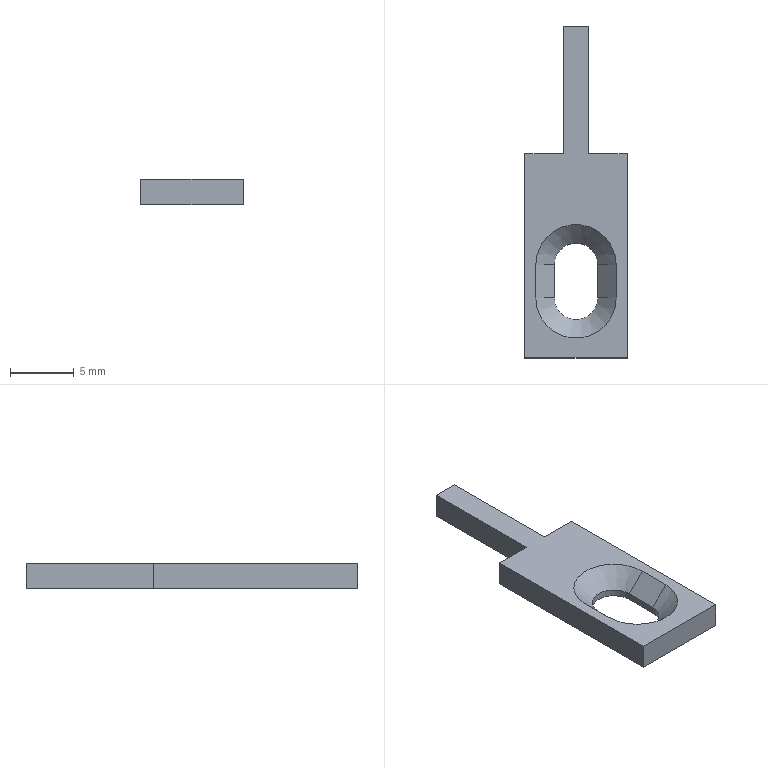Part | NX | features BREP 1 | 1 solid | 18 faces | box 8 x 26 x 2 mm | volume 240.274 mm3 | plane 14 | cone 2 | cylinder 2 | commonest cylinder face diameters 3.4 x2
STEP:
#1=CARTESIAN_POINT('',(-3.15,-3.3,2.));
#2=VERTEX_POINT('',#1);
#3=CARTESIAN_POINT('',(-1.7,-3.3,0.55));
#4=VERTEX_POINT('',#3);
#5=CARTESIAN_POINT('',(0.,-3.3,-1.15));
#6=DIRECTION('',(0.7071,0.,-0.7071));
#7=VECTOR('',#6,1000.);
#8=LINE('',#5,#7);
#9=EDGE_CURVE('',#2,#4,#8,.T.);
#10=ORIENTED_EDGE('',*,*,#9,.T.);
#11=CARTESIAN_POINT('',(-1.7,-0.7,0.55));
#12=VERTEX_POINT('',#11);
#13=CARTESIAN_POINT('',(-1.7,-0.7,0.55));
#14=DIRECTION('',(0.,-1.,0.));
#15=VECTOR('',#14,1000.);
#16=LINE('',#13,#15);
#17=EDGE_CURVE('',#12,#4,#16,.T.);
#18=ORIENTED_EDGE('',*,*,#17,.F.);
#19=CARTESIAN_POINT('',(-3.15,-0.7,2.));
#20=VERTEX_POINT('',#19);
#21=CARTESIAN_POINT('',(0.,-0.7,-1.15));
#22=DIRECTION('',(-0.7071,0.,0.7071));
#23=VECTOR('',#22,1000.);
#24=LINE('',#21,#23);
#25=EDGE_CURVE('',#12,#20,#24,.T.);
#26=ORIENTED_EDGE('',*,*,#25,.T.);
#27=CARTESIAN_POINT('',(-3.15,-0.7,2.));
#28=DIRECTION('',(0.,-1.,0.));
#29=VECTOR('',#28,1000.);
#30=LINE('',#27,#29);
#31=EDGE_CURVE('',#20,#2,#30,.T.);
#32=ORIENTED_EDGE('',*,*,#31,.T.);
#33=EDGE_LOOP('',(#10,#18,#26,#32));
#34=FACE_BOUND('',#33,.T.);
#35=CARTESIAN_POINT('',(0.,-0.7,-1.15));
#36=DIRECTION('',(-0.7071,0.,-0.7071));
#37=DIRECTION('',(-0.7071,0.,0.7071));
#38=AXIS2_PLACEMENT_3D('',#35,#36,#37);
#39=PLANE('',#38);
#40=ADVANCED_FACE('',(#34),#39,.F.);
#41=CARTESIAN_POINT('',(3.15,-3.3,2.));
#42=VERTEX_POINT('',#41);
#43=CARTESIAN_POINT('',(1.7,-3.3,0.55));
#44=VERTEX_POINT('',#43);
#45=CARTESIAN_POINT('',(1.7,-3.3,0.55));
#46=DIRECTION('',(-0.7071,0.,-0.7071));
#47=VECTOR('',#46,1000.);
#48=LINE('',#45,#47);
#49=EDGE_CURVE('',#42,#44,#48,.T.);
#50=ORIENTED_EDGE('',*,*,#49,.F.);
#51=CARTESIAN_POINT('',(3.15,-0.7,2.));
#52=VERTEX_POINT('',#51);
#53=CARTESIAN_POINT('',(3.15,-0.7,2.));
#54=DIRECTION('',(0.,-1.,0.));
#55=VECTOR('',#54,1000.);
#56=LINE('',#53,#55);
#57=EDGE_CURVE('',#52,#42,#56,.T.);
#58=ORIENTED_EDGE('',*,*,#57,.F.);
#59=CARTESIAN_POINT('',(1.7,-0.7,0.55));
#60=VERTEX_POINT('',#59);
#61=CARTESIAN_POINT('',(1.7,-0.7,0.55));
#62=DIRECTION('',(-0.7071,0.,-0.7071));
#63=VECTOR('',#62,1000.);
#64=LINE('',#61,#63);
#65=EDGE_CURVE('',#52,#60,#64,.T.);
#66=ORIENTED_EDGE('',*,*,#65,.T.);
#67=CARTESIAN_POINT('',(1.7,-0.7,0.55));
#68=DIRECTION('',(0.,-1.,0.));
#69=VECTOR('',#68,1000.);
#70=LINE('',#67,#69);
#71=EDGE_CURVE('',#60,#44,#70,.T.);
#72=ORIENTED_EDGE('',*,*,#71,.T.);
#73=EDGE_LOOP('',(#50,#58,#66,#72));
#74=FACE_BOUND('',#73,.T.);
#75=CARTESIAN_POINT('',(1.7,-0.7,0.55));
#76=DIRECTION('',(-0.7071,0.,0.7071));
#77=DIRECTION('',(0.7071,0.,0.7071));
#78=AXIS2_PLACEMENT_3D('',#75,#76,#77);
#79=PLANE('',#78);
#80=ADVANCED_FACE('',(#74),#79,.T.);
#81=CARTESIAN_POINT('',(0.,-0.7,0.55));
#82=DIRECTION('',(0.,0.,1.));
#83=DIRECTION('',(1.,0.,0.));
#84=AXIS2_PLACEMENT_3D('',#81,#82,#83);
#85=CIRCLE('',#84,1.7);
#86=EDGE_CURVE('',#60,#12,#85,.T.);
#87=ORIENTED_EDGE('',*,*,#86,.F.);
#88=ORIENTED_EDGE('',*,*,#65,.F.);
#89=CARTESIAN_POINT('',(0.,-0.7,2.));
#90=DIRECTION('',(0.,0.,1.));
#91=DIRECTION('',(1.,0.,0.));
#92=AXIS2_PLACEMENT_3D('',#89,#90,#91);
#93=CIRCLE('',#92,3.15);
#94=EDGE_CURVE('',#52,#20,#93,.T.);
#95=ORIENTED_EDGE('',*,*,#94,.T.);
#96=ORIENTED_EDGE('',*,*,#25,.F.);
#97=EDGE_LOOP('',(#87,#88,#95,#96));
#98=FACE_BOUND('',#97,.T.);
#99=CARTESIAN_POINT('',(0.,-0.7,2.));
#100=DIRECTION('',(0.,0.,1.));
#101=DIRECTION('',(1.,0.,0.));
#102=AXIS2_PLACEMENT_3D('',#99,#100,#101);
#103=CONICAL_SURFACE('',#102,3.15,0.7854);
#104=ADVANCED_FACE('',(#98),#103,.F.);
#105=CARTESIAN_POINT('',(0.,-3.3,2.));
#106=DIRECTION('',(0.,0.,1.));
#107=DIRECTION('',(1.,0.,0.));
#108=AXIS2_PLACEMENT_3D('',#105,#106,#107);
#109=CIRCLE('',#108,3.15);
#110=EDGE_CURVE('',#2,#42,#109,.T.);
#111=ORIENTED_EDGE('',*,*,#110,.T.);
#112=ORIENTED_EDGE('',*,*,#49,.T.);
#113=CARTESIAN_POINT('',(0.,-3.3,0.55));
#114=DIRECTION('',(0.,0.,1.));
#115=DIRECTION('',(1.,0.,0.));
#116=AXIS2_PLACEMENT_3D('',#113,#114,#115);
#117=CIRCLE('',#116,1.7);
#118=EDGE_CURVE('',#4,#44,#117,.T.);
#119=ORIENTED_EDGE('',*,*,#118,.F.);
#120=ORIENTED_EDGE('',*,*,#9,.F.);
#121=EDGE_LOOP('',(#111,#112,#119,#120));
#122=FACE_BOUND('',#121,.T.);
#123=CARTESIAN_POINT('',(0.,-3.3,2.));
#124=DIRECTION('',(0.,0.,1.));
#125=DIRECTION('',(1.,0.,0.));
#126=AXIS2_PLACEMENT_3D('',#123,#124,#125);
#127=CONICAL_SURFACE('',#126,3.15,0.7854);
#128=ADVANCED_FACE('',(#122),#127,.F.);
#129=CARTESIAN_POINT('',(1.7,-0.7,0.));
#130=VERTEX_POINT('',#129);
#131=CARTESIAN_POINT('',(1.7,-3.3,0.));
#132=VERTEX_POINT('',#131);
#133=CARTESIAN_POINT('',(1.7,0.,0.));
#134=DIRECTION('',(0.,-1.,0.));
#135=VECTOR('',#134,1000.);
#136=LINE('',#133,#135);
#137=EDGE_CURVE('',#130,#132,#136,.T.);
#138=ORIENTED_EDGE('',*,*,#137,.T.);
#139=CARTESIAN_POINT('',(1.7,-3.3,-16.));
#140=DIRECTION('',(0.,0.,-1.));
#141=VECTOR('',#140,1000.);
#142=LINE('',#139,#141);
#143=EDGE_CURVE('',#44,#132,#142,.T.);
#144=ORIENTED_EDGE('',*,*,#143,.F.);
#145=ORIENTED_EDGE('',*,*,#71,.F.);
#146=CARTESIAN_POINT('',(1.7,-0.7,-16.));
#147=DIRECTION('',(0.,0.,-1.));
#148=VECTOR('',#147,1000.);
#149=LINE('',#146,#148);
#150=EDGE_CURVE('',#60,#130,#149,.T.);
#151=ORIENTED_EDGE('',*,*,#150,.T.);
#152=EDGE_LOOP('',(#138,#144,#145,#151));
#153=FACE_BOUND('',#152,.T.);
#154=CARTESIAN_POINT('',(1.7,-0.7,-16.));
#155=DIRECTION('',(-1.,0.,0.));
#156=DIRECTION('',(0.,-1.,0.));
#157=AXIS2_PLACEMENT_3D('',#154,#155,#156);
#158=PLANE('',#157);
#159=ADVANCED_FACE('',(#153),#158,.T.);
#160=CARTESIAN_POINT('',(-1.7,-0.7,0.));
#161=VERTEX_POINT('',#160);
#162=CARTESIAN_POINT('',(-1.7,-0.7,2.));
#163=DIRECTION('',(0.,0.,1.));
#164=VECTOR('',#163,1000.);
#165=LINE('',#162,#164);
#166=EDGE_CURVE('',#161,#12,#165,.T.);
#167=ORIENTED_EDGE('',*,*,#166,.T.);
#168=ORIENTED_EDGE('',*,*,#17,.T.);
#169=CARTESIAN_POINT('',(-1.7,-3.3,0.));
#170=VERTEX_POINT('',#169);
#171=CARTESIAN_POINT('',(-1.7,-3.3,2.));
#172=DIRECTION('',(0.,0.,-1.));
#173=VECTOR('',#172,1000.);
#174=LINE('',#171,#173);
#175=EDGE_CURVE('',#4,#170,#174,.T.);
#176=ORIENTED_EDGE('',*,*,#175,.T.);
#177=CARTESIAN_POINT('',(-1.7,0.,0.));
#178=DIRECTION('',(0.,-1.,0.));
#179=VECTOR('',#178,1000.);
#180=LINE('',#177,#179);
#181=EDGE_CURVE('',#161,#170,#180,.T.);
#182=ORIENTED_EDGE('',*,*,#181,.F.);
#183=EDGE_LOOP('',(#167,#168,#176,#182));
#184=FACE_BOUND('',#183,.T.);
#185=CARTESIAN_POINT('',(-1.7,-0.7,2.));
#186=DIRECTION('',(-1.,0.,0.));
#187=DIRECTION('',(0.,-1.,0.));
#188=AXIS2_PLACEMENT_3D('',#185,#186,#187);
#189=PLANE('',#188);
#190=ADVANCED_FACE('',(#184),#189,.F.);
#191=ORIENTED_EDGE('',*,*,#175,.F.);
#192=ORIENTED_EDGE('',*,*,#118,.T.);
#193=ORIENTED_EDGE('',*,*,#143,.T.);
#194=CARTESIAN_POINT('',(0.,-3.3,0.));
#195=DIRECTION('',(0.,0.,1.));
#196=DIRECTION('',(1.,0.,0.));
#197=AXIS2_PLACEMENT_3D('',#194,#195,#196);
#198=CIRCLE('',#197,1.7);
#199=EDGE_CURVE('',#170,#132,#198,.T.);
#200=ORIENTED_EDGE('',*,*,#199,.F.);
#201=EDGE_LOOP('',(#191,#192,#193,#200));
#202=FACE_BOUND('',#201,.T.);
#203=CARTESIAN_POINT('',(0.,-3.3,2.));
#204=DIRECTION('',(0.,0.,1.));
#205=DIRECTION('',(1.,0.,0.));
#206=AXIS2_PLACEMENT_3D('',#203,#204,#205);
#207=CYLINDRICAL_SURFACE('',#206,1.7);
#208=ADVANCED_FACE('',(#202),#207,.F.);
#209=ORIENTED_EDGE('',*,*,#150,.F.);
#210=ORIENTED_EDGE('',*,*,#86,.T.);
#211=ORIENTED_EDGE('',*,*,#166,.F.);
#212=CARTESIAN_POINT('',(0.,-0.7,0.));
#213=DIRECTION('',(0.,0.,1.));
#214=DIRECTION('',(1.,0.,0.));
#215=AXIS2_PLACEMENT_3D('',#212,#213,#214);
#216=CIRCLE('',#215,1.7);
#217=EDGE_CURVE('',#130,#161,#216,.T.);
#218=ORIENTED_EDGE('',*,*,#217,.F.);
#219=EDGE_LOOP('',(#209,#210,#211,#218));
#220=FACE_BOUND('',#219,.T.);
#221=CARTESIAN_POINT('',(0.,-0.7,2.));
#222=DIRECTION('',(0.,0.,1.));
#223=DIRECTION('',(1.,0.,0.));
#224=AXIS2_PLACEMENT_3D('',#221,#222,#223);
#225=CYLINDRICAL_SURFACE('',#224,1.7);
#226=ADVANCED_FACE('',(#220),#225,.F.);
#227=CARTESIAN_POINT('',(4.,8.,0.));
#228=VERTEX_POINT('',#227);
#229=CARTESIAN_POINT('',(1.,8.,0.));
#230=VERTEX_POINT('',#229);
#231=CARTESIAN_POINT('',(1.,8.,0.));
#232=DIRECTION('',(-1.,0.,0.));
#233=VECTOR('',#232,1000.);
#234=LINE('',#231,#233);
#235=EDGE_CURVE('',#228,#230,#234,.T.);
#236=ORIENTED_EDGE('',*,*,#235,.F.);
#237=CARTESIAN_POINT('',(4.,-8.,0.));
#238=VERTEX_POINT('',#237);
#239=CARTESIAN_POINT('',(4.,-8.,0.));
#240=DIRECTION('',(0.,1.,0.));
#241=VECTOR('',#240,1000.);
#242=LINE('',#239,#241);
#243=EDGE_CURVE('',#238,#228,#242,.T.);
#244=ORIENTED_EDGE('',*,*,#243,.F.);
#245=CARTESIAN_POINT('',(-4.,-8.,0.));
#246=VERTEX_POINT('',#245);
#247=CARTESIAN_POINT('',(-4.,-8.,0.));
#248=DIRECTION('',(1.,0.,0.));
#249=VECTOR('',#248,1000.);
#250=LINE('',#247,#249);
#251=EDGE_CURVE('',#246,#238,#250,.T.);
#252=ORIENTED_EDGE('',*,*,#251,.F.);
#253=CARTESIAN_POINT('',(-4.,8.,0.));
#254=VERTEX_POINT('',#253);
#255=CARTESIAN_POINT('',(-4.,-8.,0.));
#256=DIRECTION('',(0.,-1.,0.));
#257=VECTOR('',#256,1000.);
#258=LINE('',#255,#257);
#259=EDGE_CURVE('',#254,#246,#258,.T.);
#260=ORIENTED_EDGE('',*,*,#259,.F.);
#261=CARTESIAN_POINT('',(-1.,8.,0.));
#262=VERTEX_POINT('',#261);
#263=CARTESIAN_POINT('',(-4.,8.,0.));
#264=DIRECTION('',(-1.,0.,0.));
#265=VECTOR('',#264,1000.);
#266=LINE('',#263,#265);
#267=EDGE_CURVE('',#262,#254,#266,.T.);
#268=ORIENTED_EDGE('',*,*,#267,.F.);
#269=CARTESIAN_POINT('',(-1.,18.,0.));
#270=VERTEX_POINT('',#269);
#271=CARTESIAN_POINT('',(-1.,18.,0.));
#272=DIRECTION('',(0.,-1.,0.));
#273=VECTOR('',#272,1000.);
#274=LINE('',#271,#273);
#275=EDGE_CURVE('',#270,#262,#274,.T.);
#276=ORIENTED_EDGE('',*,*,#275,.F.);
#277=CARTESIAN_POINT('',(1.,18.,0.));
#278=VERTEX_POINT('',#277);
#279=CARTESIAN_POINT('',(1.,18.,0.));
#280=DIRECTION('',(-1.,0.,0.));
#281=VECTOR('',#280,1000.);
#282=LINE('',#279,#281);
#283=EDGE_CURVE('',#278,#270,#282,.T.);
#284=ORIENTED_EDGE('',*,*,#283,.F.);
#285=CARTESIAN_POINT('',(1.,18.,0.));
#286=DIRECTION('',(0.,1.,0.));
#287=VECTOR('',#286,1000.);
#288=LINE('',#285,#287);
#289=EDGE_CURVE('',#230,#278,#288,.T.);
#290=ORIENTED_EDGE('',*,*,#289,.F.);
#291=EDGE_LOOP('',(#236,#244,#252,#260,#268,#276,#284,#290));
#292=FACE_BOUND('',#291,.T.);
#293=ORIENTED_EDGE('',*,*,#217,.T.);
#294=ORIENTED_EDGE('',*,*,#181,.T.);
#295=ORIENTED_EDGE('',*,*,#199,.T.);
#296=ORIENTED_EDGE('',*,*,#137,.F.);
#297=EDGE_LOOP('',(#293,#294,#295,#296));
#298=FACE_BOUND('',#297,.T.);
#299=CARTESIAN_POINT('',(0.,0.,0.));
#300=DIRECTION('',(0.,0.,1.));
#301=DIRECTION('',(1.,0.,0.));
#302=AXIS2_PLACEMENT_3D('',#299,#300,#301);
#303=PLANE('',#302);
#304=ADVANCED_FACE('',(#292,#298),#303,.F.);
#305=CARTESIAN_POINT('',(4.,8.,2.));
#306=VERTEX_POINT('',#305);
#307=CARTESIAN_POINT('',(1.,8.,2.));
#308=VERTEX_POINT('',#307);
#309=CARTESIAN_POINT('',(1.,8.,2.));
#310=DIRECTION('',(-1.,0.,0.));
#311=VECTOR('',#310,1000.);
#312=LINE('',#309,#311);
#313=EDGE_CURVE('',#306,#308,#312,.T.);
#314=ORIENTED_EDGE('',*,*,#313,.T.);
#315=CARTESIAN_POINT('',(1.,18.,2.));
#316=VERTEX_POINT('',#315);
#317=CARTESIAN_POINT('',(1.,18.,2.));
#318=DIRECTION('',(0.,1.,0.));
#319=VECTOR('',#318,1000.);
#320=LINE('',#317,#319);
#321=EDGE_CURVE('',#308,#316,#320,.T.);
#322=ORIENTED_EDGE('',*,*,#321,.T.);
#323=CARTESIAN_POINT('',(-1.,18.,2.));
#324=VERTEX_POINT('',#323);
#325=CARTESIAN_POINT('',(1.,18.,2.));
#326=DIRECTION('',(-1.,0.,0.));
#327=VECTOR('',#326,1000.);
#328=LINE('',#325,#327);
#329=EDGE_CURVE('',#316,#324,#328,.T.);
#330=ORIENTED_EDGE('',*,*,#329,.T.);
#331=CARTESIAN_POINT('',(-1.,8.,2.));
#332=VERTEX_POINT('',#331);
#333=CARTESIAN_POINT('',(-1.,18.,2.));
#334=DIRECTION('',(0.,-1.,0.));
#335=VECTOR('',#334,1000.);
#336=LINE('',#333,#335);
#337=EDGE_CURVE('',#324,#332,#336,.T.);
#338=ORIENTED_EDGE('',*,*,#337,.T.);
#339=CARTESIAN_POINT('',(-4.,8.,2.));
#340=VERTEX_POINT('',#339);
#341=CARTESIAN_POINT('',(-4.,8.,2.));
#342=DIRECTION('',(-1.,0.,0.));
#343=VECTOR('',#342,1000.);
#344=LINE('',#341,#343);
#345=EDGE_CURVE('',#332,#340,#344,.T.);
#346=ORIENTED_EDGE('',*,*,#345,.T.);
#347=CARTESIAN_POINT('',(-4.,-8.,2.));
#348=VERTEX_POINT('',#347);
#349=CARTESIAN_POINT('',(-4.,-8.,2.));
#350=DIRECTION('',(0.,-1.,0.));
#351=VECTOR('',#350,1000.);
#352=LINE('',#349,#351);
#353=EDGE_CURVE('',#340,#348,#352,.T.);
#354=ORIENTED_EDGE('',*,*,#353,.T.);
#355=CARTESIAN_POINT('',(4.,-8.,2.));
#356=VERTEX_POINT('',#355);
#357=CARTESIAN_POINT('',(-4.,-8.,2.));
#358=DIRECTION('',(1.,0.,0.));
#359=VECTOR('',#358,1000.);
#360=LINE('',#357,#359);
#361=EDGE_CURVE('',#348,#356,#360,.T.);
#362=ORIENTED_EDGE('',*,*,#361,.T.);
#363=CARTESIAN_POINT('',(4.,-8.,2.));
#364=DIRECTION('',(0.,1.,0.));
#365=VECTOR('',#364,1000.);
#366=LINE('',#363,#365);
#367=EDGE_CURVE('',#356,#306,#366,.T.);
#368=ORIENTED_EDGE('',*,*,#367,.T.);
#369=EDGE_LOOP('',(#314,#322,#330,#338,#346,#354,#362,#368));
#370=FACE_BOUND('',#369,.T.);
#371=ORIENTED_EDGE('',*,*,#31,.F.);
#372=ORIENTED_EDGE('',*,*,#94,.F.);
#373=ORIENTED_EDGE('',*,*,#57,.T.);
#374=ORIENTED_EDGE('',*,*,#110,.F.);
#375=EDGE_LOOP('',(#371,#372,#373,#374));
#376=FACE_BOUND('',#375,.T.);
#377=CARTESIAN_POINT('',(0.,0.,2.));
#378=DIRECTION('',(0.,0.,1.));
#379=DIRECTION('',(1.,0.,0.));
#380=AXIS2_PLACEMENT_3D('',#377,#378,#379);
#381=PLANE('',#380);
#382=ADVANCED_FACE('',(#370,#376),#381,.T.);
#383=ORIENTED_EDGE('',*,*,#243,.T.);
#384=CARTESIAN_POINT('',(4.,8.,2.));
#385=DIRECTION('',(0.,0.,-1.));
#386=VECTOR('',#385,1000.);
#387=LINE('',#384,#386);
#388=EDGE_CURVE('',#306,#228,#387,.T.);
#389=ORIENTED_EDGE('',*,*,#388,.F.);
#390=ORIENTED_EDGE('',*,*,#367,.F.);
#391=CARTESIAN_POINT('',(4.,-8.,2.));
#392=DIRECTION('',(0.,0.,-1.));
#393=VECTOR('',#392,1000.);
#394=LINE('',#391,#393);
#395=EDGE_CURVE('',#356,#238,#394,.T.);
#396=ORIENTED_EDGE('',*,*,#395,.T.);
#397=EDGE_LOOP('',(#383,#389,#390,#396));
#398=FACE_BOUND('',#397,.T.);
#399=CARTESIAN_POINT('',(4.,-8.,2.));
#400=DIRECTION('',(-1.,0.,0.));
#401=DIRECTION('',(0.,0.,1.));
#402=AXIS2_PLACEMENT_3D('',#399,#400,#401);
#403=PLANE('',#402);
#404=ADVANCED_FACE('',(#398),#403,.F.);
#405=ORIENTED_EDGE('',*,*,#251,.T.);
#406=ORIENTED_EDGE('',*,*,#395,.F.);
#407=ORIENTED_EDGE('',*,*,#361,.F.);
#408=CARTESIAN_POINT('',(-4.,-8.,2.));
#409=DIRECTION('',(0.,0.,-1.));
#410=VECTOR('',#409,1000.);
#411=LINE('',#408,#410);
#412=EDGE_CURVE('',#348,#246,#411,.T.);
#413=ORIENTED_EDGE('',*,*,#412,.T.);
#414=EDGE_LOOP('',(#405,#406,#407,#413));
#415=FACE_BOUND('',#414,.T.);
#416=CARTESIAN_POINT('',(-4.,-8.,2.));
#417=DIRECTION('',(0.,1.,0.));
#418=DIRECTION('',(0.,0.,1.));
#419=AXIS2_PLACEMENT_3D('',#416,#417,#418);
#420=PLANE('',#419);
#421=ADVANCED_FACE('',(#415),#420,.F.);
#422=ORIENTED_EDGE('',*,*,#259,.T.);
#423=ORIENTED_EDGE('',*,*,#412,.F.);
#424=ORIENTED_EDGE('',*,*,#353,.F.);
#425=CARTESIAN_POINT('',(-4.,8.,2.));
#426=DIRECTION('',(0.,0.,-1.));
#427=VECTOR('',#426,1000.);
#428=LINE('',#425,#427);
#429=EDGE_CURVE('',#340,#254,#428,.T.);
#430=ORIENTED_EDGE('',*,*,#429,.T.);
#431=EDGE_LOOP('',(#422,#423,#424,#430));
#432=FACE_BOUND('',#431,.T.);
#433=CARTESIAN_POINT('',(-4.,-8.,2.));
#434=DIRECTION('',(1.,0.,0.));
#435=DIRECTION('',(0.,0.,-1.));
#436=AXIS2_PLACEMENT_3D('',#433,#434,#435);
#437=PLANE('',#436);
#438=ADVANCED_FACE('',(#432),#437,.F.);
#439=ORIENTED_EDGE('',*,*,#267,.T.);
#440=ORIENTED_EDGE('',*,*,#429,.F.);
#441=ORIENTED_EDGE('',*,*,#345,.F.);
#442=CARTESIAN_POINT('',(-1.,8.,2.));
#443=DIRECTION('',(0.,0.,-1.));
#444=VECTOR('',#443,1000.);
#445=LINE('',#442,#444);
#446=EDGE_CURVE('',#332,#262,#445,.T.);
#447=ORIENTED_EDGE('',*,*,#446,.T.);
#448=EDGE_LOOP('',(#439,#440,#441,#447));
#449=FACE_BOUND('',#448,.T.);
#450=CARTESIAN_POINT('',(-4.,8.,2.));
#451=DIRECTION('',(0.,-1.,0.));
#452=DIRECTION('',(1.,0.,0.));
#453=AXIS2_PLACEMENT_3D('',#450,#451,#452);
#454=PLANE('',#453);
#455=ADVANCED_FACE('',(#449),#454,.F.);
#456=ORIENTED_EDGE('',*,*,#275,.T.);
#457=ORIENTED_EDGE('',*,*,#446,.F.);
#458=ORIENTED_EDGE('',*,*,#337,.F.);
#459=CARTESIAN_POINT('',(-1.,18.,2.));
#460=DIRECTION('',(0.,0.,-1.));
#461=VECTOR('',#460,1000.);
#462=LINE('',#459,#461);
#463=EDGE_CURVE('',#324,#270,#462,.T.);
#464=ORIENTED_EDGE('',*,*,#463,.T.);
#465=EDGE_LOOP('',(#456,#457,#458,#464));
#466=FACE_BOUND('',#465,.T.);
#467=CARTESIAN_POINT('',(-1.,18.,2.));
#468=DIRECTION('',(1.,0.,0.));
#469=DIRECTION('',(0.,1.,0.));
#470=AXIS2_PLACEMENT_3D('',#467,#468,#469);
#471=PLANE('',#470);
#472=ADVANCED_FACE('',(#466),#471,.F.);
#473=ORIENTED_EDGE('',*,*,#283,.T.);
#474=ORIENTED_EDGE('',*,*,#463,.F.);
#475=ORIENTED_EDGE('',*,*,#329,.F.);
#476=CARTESIAN_POINT('',(1.,18.,2.));
#477=DIRECTION('',(0.,0.,-1.));
#478=VECTOR('',#477,1000.);
#479=LINE('',#476,#478);
#480=EDGE_CURVE('',#316,#278,#479,.T.);
#481=ORIENTED_EDGE('',*,*,#480,.T.);
#482=EDGE_LOOP('',(#473,#474,#475,#481));
#483=FACE_BOUND('',#482,.T.);
#484=CARTESIAN_POINT('',(1.,18.,2.));
#485=DIRECTION('',(0.,-1.,0.));
#486=DIRECTION('',(0.,0.,-1.));
#487=AXIS2_PLACEMENT_3D('',#484,#485,#486);
#488=PLANE('',#487);
#489=ADVANCED_FACE('',(#483),#488,.F.);
#490=ORIENTED_EDGE('',*,*,#289,.T.);
#491=ORIENTED_EDGE('',*,*,#480,.F.);
#492=ORIENTED_EDGE('',*,*,#321,.F.);
#493=CARTESIAN_POINT('',(1.,8.,2.));
#494=DIRECTION('',(0.,0.,-1.));
#495=VECTOR('',#494,1000.);
#496=LINE('',#493,#495);
#497=EDGE_CURVE('',#308,#230,#496,.T.);
#498=ORIENTED_EDGE('',*,*,#497,.T.);
#499=EDGE_LOOP('',(#490,#491,#492,#498));
#500=FACE_BOUND('',#499,.T.);
#501=CARTESIAN_POINT('',(1.,18.,2.));
#502=DIRECTION('',(-1.,0.,0.));
#503=DIRECTION('',(0.,-1.,0.));
#504=AXIS2_PLACEMENT_3D('',#501,#502,#503);
#505=PLANE('',#504);
#506=ADVANCED_FACE('',(#500),#505,.F.);
#507=ORIENTED_EDGE('',*,*,#235,.T.);
#508=ORIENTED_EDGE('',*,*,#497,.F.);
#509=ORIENTED_EDGE('',*,*,#313,.F.);
#510=ORIENTED_EDGE('',*,*,#388,.T.);
#511=EDGE_LOOP('',(#507,#508,#509,#510));
#512=FACE_BOUND('',#511,.T.);
#513=CARTESIAN_POINT('',(1.,8.,2.));
#514=DIRECTION('',(0.,-1.,0.));
#515=DIRECTION('',(1.,0.,0.));
#516=AXIS2_PLACEMENT_3D('',#513,#514,#515);
#517=PLANE('',#516);
#518=ADVANCED_FACE('',(#512),#517,.F.);
#519=CLOSED_SHELL('',(#40,#80,#104,#128,#159,#190,#208,#226,#304,#382,#404,#421,#438,#455,#472,#489,#506,#518));
#520=MANIFOLD_SOLID_BREP('',#519);
#521=(LENGTH_UNIT()NAMED_UNIT(*)SI_UNIT(.MILLI.,.METRE.));
#522=UNCERTAINTY_MEASURE_WITH_UNIT(LENGTH_MEASURE(0.00001),#521,'','');
#523=(NAMED_UNIT(*)PLANE_ANGLE_UNIT()SI_UNIT($,.RADIAN.));
#524=(NAMED_UNIT(*)SI_UNIT($,.STERADIAN.)SOLID_ANGLE_UNIT());
#525=(GEOMETRIC_REPRESENTATION_CONTEXT(3)GLOBAL_UNCERTAINTY_ASSIGNED_CONTEXT((#522))GLOBAL_UNIT_ASSIGNED_CONTEXT((#521,#523,#524))REPRESENTATION_CONTEXT('',''));
#526=ADVANCED_BREP_SHAPE_REPRESENTATION('',(#520),#525);